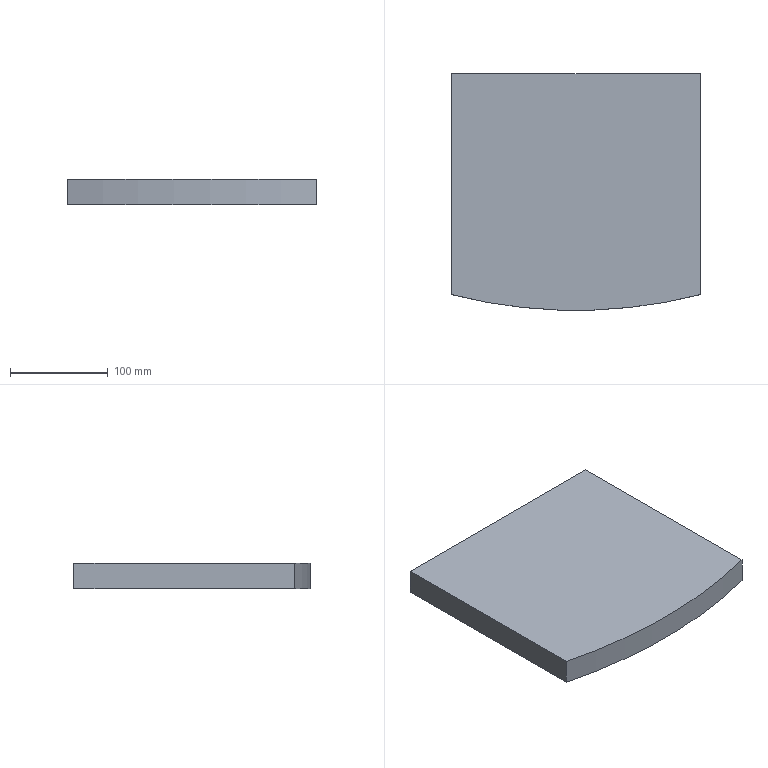Part | SolidWorks | features Extrusion 1 | 1 solid | 6 faces | box 254 x 241.3 x 26 mm | volume 1558264 mm3 | plane 5 | cylinder 1 | commonest cylinder face diameters 1016 x1
STEP:
#1=CARTESIAN_POINT('',(-127.,152.4,-13.));
#2=VERTEX_POINT('',#1);
#3=CARTESIAN_POINT('',(-127.,-72.769,-13.));
#4=VERTEX_POINT('',#3);
#5=CARTESIAN_POINT('',(-127.,152.4,-13.));
#6=DIRECTION('',(0.,-1.,0.));
#7=VECTOR('',#6,1000.);
#8=LINE('',#5,#7);
#9=EDGE_CURVE('',#2,#4,#8,.T.);
#10=ORIENTED_EDGE('',*,*,#9,.T.);
#11=CARTESIAN_POINT('',(-127.,-72.769,13.));
#12=VERTEX_POINT('',#11);
#13=CARTESIAN_POINT('',(-127.,-72.769,13.));
#14=DIRECTION('',(0.,0.,-1.));
#15=VECTOR('',#14,1000.);
#16=LINE('',#13,#15);
#17=EDGE_CURVE('',#12,#4,#16,.T.);
#18=ORIENTED_EDGE('',*,*,#17,.F.);
#19=CARTESIAN_POINT('',(-127.,152.4,13.));
#20=VERTEX_POINT('',#19);
#21=CARTESIAN_POINT('',(-127.,152.4,13.));
#22=DIRECTION('',(0.,-1.,0.));
#23=VECTOR('',#22,1000.);
#24=LINE('',#21,#23);
#25=EDGE_CURVE('',#20,#12,#24,.T.);
#26=ORIENTED_EDGE('',*,*,#25,.F.);
#27=CARTESIAN_POINT('',(-127.,152.4,13.));
#28=DIRECTION('',(0.,0.,-1.));
#29=VECTOR('',#28,1000.);
#30=LINE('',#27,#29);
#31=EDGE_CURVE('',#20,#2,#30,.T.);
#32=ORIENTED_EDGE('',*,*,#31,.T.);
#33=EDGE_LOOP('',(#10,#18,#26,#32));
#34=FACE_OUTER_BOUND('',#33,.T.);
#35=CARTESIAN_POINT('',(-127.,152.4,13.));
#36=DIRECTION('',(1.,0.,0.));
#37=DIRECTION('',(0.,1.,0.));
#38=AXIS2_PLACEMENT_3D('',#35,#36,#37);
#39=PLANE('',#38);
#40=ADVANCED_FACE('',(#34),#39,.F.);
#41=CARTESIAN_POINT('',(127.,-72.769,-13.));
#42=VERTEX_POINT('',#41);
#43=CARTESIAN_POINT('',(0.,419.1,-13.));
#44=DIRECTION('',(0.,0.,1.));
#45=DIRECTION('',(1.,0.,0.));
#46=AXIS2_PLACEMENT_3D('',#43,#44,#45);
#47=CIRCLE('',#46,508.);
#48=EDGE_CURVE('',#4,#42,#47,.T.);
#49=ORIENTED_EDGE('',*,*,#48,.T.);
#50=CARTESIAN_POINT('',(127.,-72.769,13.));
#51=VERTEX_POINT('',#50);
#52=CARTESIAN_POINT('',(127.,-72.769,13.));
#53=DIRECTION('',(0.,0.,-1.));
#54=VECTOR('',#53,1000.);
#55=LINE('',#52,#54);
#56=EDGE_CURVE('',#51,#42,#55,.T.);
#57=ORIENTED_EDGE('',*,*,#56,.F.);
#58=CARTESIAN_POINT('',(0.,419.1,13.));
#59=DIRECTION('',(0.,0.,1.));
#60=DIRECTION('',(1.,0.,0.));
#61=AXIS2_PLACEMENT_3D('',#58,#59,#60);
#62=CIRCLE('',#61,508.);
#63=EDGE_CURVE('',#12,#51,#62,.T.);
#64=ORIENTED_EDGE('',*,*,#63,.F.);
#65=ORIENTED_EDGE('',*,*,#17,.T.);
#66=EDGE_LOOP('',(#49,#57,#64,#65));
#67=FACE_OUTER_BOUND('',#66,.T.);
#68=CARTESIAN_POINT('',(0.,419.1,13.));
#69=DIRECTION('',(0.,0.,-1.));
#70=DIRECTION('',(-1.,0.,0.));
#71=AXIS2_PLACEMENT_3D('',#68,#69,#70);
#72=CYLINDRICAL_SURFACE('',#71,508.);
#73=ADVANCED_FACE('',(#67),#72,.T.);
#74=CARTESIAN_POINT('',(127.,152.4,-13.));
#75=VERTEX_POINT('',#74);
#76=CARTESIAN_POINT('',(127.,152.4,-13.));
#77=DIRECTION('',(0.,1.,0.));
#78=VECTOR('',#77,1000.);
#79=LINE('',#76,#78);
#80=EDGE_CURVE('',#42,#75,#79,.T.);
#81=ORIENTED_EDGE('',*,*,#80,.T.);
#82=CARTESIAN_POINT('',(127.,152.4,13.));
#83=VERTEX_POINT('',#82);
#84=CARTESIAN_POINT('',(127.,152.4,13.));
#85=DIRECTION('',(0.,0.,-1.));
#86=VECTOR('',#85,1000.);
#87=LINE('',#84,#86);
#88=EDGE_CURVE('',#83,#75,#87,.T.);
#89=ORIENTED_EDGE('',*,*,#88,.F.);
#90=CARTESIAN_POINT('',(127.,152.4,13.));
#91=DIRECTION('',(0.,1.,0.));
#92=VECTOR('',#91,1000.);
#93=LINE('',#90,#92);
#94=EDGE_CURVE('',#51,#83,#93,.T.);
#95=ORIENTED_EDGE('',*,*,#94,.F.);
#96=ORIENTED_EDGE('',*,*,#56,.T.);
#97=EDGE_LOOP('',(#81,#89,#95,#96));
#98=FACE_OUTER_BOUND('',#97,.T.);
#99=CARTESIAN_POINT('',(127.,152.4,13.));
#100=DIRECTION('',(-1.,0.,0.));
#101=DIRECTION('',(0.,0.,1.));
#102=AXIS2_PLACEMENT_3D('',#99,#100,#101);
#103=PLANE('',#102);
#104=ADVANCED_FACE('',(#98),#103,.F.);
#105=CARTESIAN_POINT('',(-127.,152.4,-13.));
#106=DIRECTION('',(-1.,0.,0.));
#107=VECTOR('',#106,1000.);
#108=LINE('',#105,#107);
#109=EDGE_CURVE('',#75,#2,#108,.T.);
#110=ORIENTED_EDGE('',*,*,#109,.T.);
#111=ORIENTED_EDGE('',*,*,#31,.F.);
#112=CARTESIAN_POINT('',(-127.,152.4,13.));
#113=DIRECTION('',(-1.,0.,0.));
#114=VECTOR('',#113,1000.);
#115=LINE('',#112,#114);
#116=EDGE_CURVE('',#83,#20,#115,.T.);
#117=ORIENTED_EDGE('',*,*,#116,.F.);
#118=ORIENTED_EDGE('',*,*,#88,.T.);
#119=EDGE_LOOP('',(#110,#111,#117,#118));
#120=FACE_OUTER_BOUND('',#119,.T.);
#121=CARTESIAN_POINT('',(-127.,152.4,13.));
#122=DIRECTION('',(0.,-1.,0.));
#123=DIRECTION('',(0.,0.,-1.));
#124=AXIS2_PLACEMENT_3D('',#121,#122,#123);
#125=PLANE('',#124);
#126=ADVANCED_FACE('',(#120),#125,.F.);
#127=ORIENTED_EDGE('',*,*,#25,.T.);
#128=ORIENTED_EDGE('',*,*,#63,.T.);
#129=ORIENTED_EDGE('',*,*,#94,.T.);
#130=ORIENTED_EDGE('',*,*,#116,.T.);
#131=EDGE_LOOP('',(#127,#128,#129,#130));
#132=FACE_OUTER_BOUND('',#131,.T.);
#133=CARTESIAN_POINT('',(0.,419.1,13.));
#134=DIRECTION('',(0.,0.,1.));
#135=DIRECTION('',(1.,0.,0.));
#136=AXIS2_PLACEMENT_3D('',#133,#134,#135);
#137=PLANE('',#136);
#138=ADVANCED_FACE('',(#132),#137,.T.);
#139=ORIENTED_EDGE('',*,*,#9,.F.);
#140=ORIENTED_EDGE('',*,*,#109,.F.);
#141=ORIENTED_EDGE('',*,*,#80,.F.);
#142=ORIENTED_EDGE('',*,*,#48,.F.);
#143=EDGE_LOOP('',(#139,#140,#141,#142));
#144=FACE_OUTER_BOUND('',#143,.T.);
#145=CARTESIAN_POINT('',(0.,419.1,-13.));
#146=DIRECTION('',(0.,0.,1.));
#147=DIRECTION('',(1.,0.,0.));
#148=AXIS2_PLACEMENT_3D('',#145,#146,#147);
#149=PLANE('',#148);
#150=ADVANCED_FACE('',(#144),#149,.F.);
#151=CLOSED_SHELL('',(#40,#73,#104,#126,#138,#150));
#152=MANIFOLD_SOLID_BREP('',#151);
#153=CARTESIAN_POINT('',(0.,0.,0.));
#154=DIRECTION('',(0.,0.,1.));
#155=DIRECTION('',(1.,0.,0.));
#156=AXIS2_PLACEMENT_3D('',#153,#154,#155);
#157=(LENGTH_UNIT()NAMED_UNIT(*)SI_UNIT(.MILLI.,.METRE.));
#158=UNCERTAINTY_MEASURE_WITH_UNIT(LENGTH_MEASURE(0.00001),#157,'','');
#159=(NAMED_UNIT(*)PLANE_ANGLE_UNIT()SI_UNIT($,.RADIAN.));
#160=(NAMED_UNIT(*)SI_UNIT($,.STERADIAN.)SOLID_ANGLE_UNIT());
#161=(GEOMETRIC_REPRESENTATION_CONTEXT(3)GLOBAL_UNCERTAINTY_ASSIGNED_CONTEXT((#158))GLOBAL_UNIT_ASSIGNED_CONTEXT((#157,#159,#160))REPRESENTATION_CONTEXT('',''));
#162=ADVANCED_BREP_SHAPE_REPRESENTATION('',(#152,#156),#161);